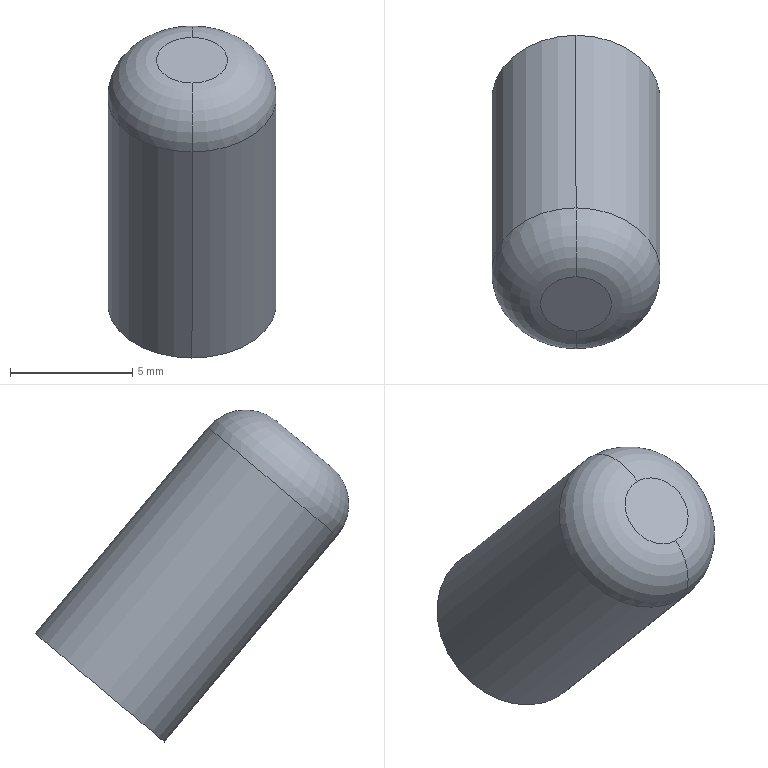Part | SolidWorks | features BaseBody 1 | 1 solid | 6 faces | box 6.9 x 12.824 x 13.576 mm | volume 469.908 mm3 | plane 2 | cylinder 2 | torus 2 | commonest cylinder face diameters 6.9 x2
STEP:
#1=CARTESIAN_POINT('',(-684.451,655.359,355.099));
#2=VERTEX_POINT('',#1);
#3=CARTESIAN_POINT('',(-684.451,660.644,359.534));
#4=VERTEX_POINT('',#3);
#5=CARTESIAN_POINT('',(-684.451,658.001,357.316));
#6=DIRECTION('',(0.000000993,-0.6428,0.766));
#7=DIRECTION('',(0.000001183,-0.766,-0.6428));
#8=AXIS2_PLACEMENT_3D('',#5,#6,#7);
#9=CIRCLE('',#8,3.45);
#10=EDGE_CURVE('',#2,#4,#9,.T.);
#11=ORIENTED_EDGE('',*,*,#10,.F.);
#12=CARTESIAN_POINT('',(-684.451,658.001,357.316));
#13=DIRECTION('',(0.000000993,-0.6428,0.766));
#14=DIRECTION('',(-0.000001183,0.766,0.6428));
#15=AXIS2_PLACEMENT_3D('',#12,#13,#14);
#16=CIRCLE('',#15,3.45);
#17=EDGE_CURVE('',#4,#2,#16,.T.);
#18=ORIENTED_EDGE('',*,*,#17,.F.);
#19=EDGE_LOOP('',(#11,#18));
#20=FACE_OUTER_BOUND('',#19,.T.);
#21=CARTESIAN_POINT('',(-750.729,655.382,355.118));
#22=DIRECTION('',(-0.000000993,0.6428,-0.766));
#23=DIRECTION('',(0.000001183,-0.766,-0.6428));
#24=AXIS2_PLACEMENT_3D('',#21,#22,#23);
#25=PLANE('',#24);
#26=ADVANCED_FACE('',(#20),#25,.T.);
#27=ORIENTED_EDGE('',*,*,#17,.T.);
#28=CARTESIAN_POINT('',(-684.451,648.288,363.525));
#29=VERTEX_POINT('',#28);
#30=CARTESIAN_POINT('',(-684.451,655.359,355.099));
#31=DIRECTION('',(0.000000993,-0.6428,0.766));
#32=VECTOR('',#31,1000.);
#33=LINE('',#30,#32);
#34=EDGE_CURVE('',#2,#29,#33,.T.);
#35=ORIENTED_EDGE('',*,*,#34,.T.);
#36=CARTESIAN_POINT('',(-684.451,653.574,367.96));
#37=VERTEX_POINT('',#36);
#38=CARTESIAN_POINT('',(-684.451,650.931,365.743));
#39=DIRECTION('',(-0.000000993,0.6428,-0.766));
#40=DIRECTION('',(0.000001183,-0.766,-0.6428));
#41=AXIS2_PLACEMENT_3D('',#38,#39,#40);
#42=CIRCLE('',#41,3.45);
#43=EDGE_CURVE('',#29,#37,#42,.T.);
#44=ORIENTED_EDGE('',*,*,#43,.T.);
#45=CARTESIAN_POINT('',(-684.451,653.574,367.96));
#46=DIRECTION('',(-0.000000993,0.6428,-0.766));
#47=VECTOR('',#46,1000.);
#48=LINE('',#45,#47);
#49=EDGE_CURVE('',#37,#4,#48,.T.);
#50=ORIENTED_EDGE('',*,*,#49,.T.);
#51=EDGE_LOOP('',(#27,#35,#44,#50));
#52=FACE_OUTER_BOUND('',#51,.T.);
#53=CARTESIAN_POINT('',(-684.451,658.001,357.316));
#54=DIRECTION('',(-0.000000993,0.6428,-0.766));
#55=DIRECTION('',(0.000001183,-0.766,-0.6428));
#56=AXIS2_PLACEMENT_3D('',#53,#54,#55);
#57=CYLINDRICAL_SURFACE('',#56,3.45);
#58=ADVANCED_FACE('',(#52),#57,.T.);
#59=ORIENTED_EDGE('',*,*,#10,.T.);
#60=ORIENTED_EDGE('',*,*,#49,.F.);
#61=CARTESIAN_POINT('',(-684.451,650.931,365.743));
#62=DIRECTION('',(-0.000000993,0.6428,-0.766));
#63=DIRECTION('',(-0.000001183,0.766,0.6428));
#64=AXIS2_PLACEMENT_3D('',#61,#62,#63);
#65=CIRCLE('',#64,3.45);
#66=EDGE_CURVE('',#37,#29,#65,.T.);
#67=ORIENTED_EDGE('',*,*,#66,.T.);
#68=ORIENTED_EDGE('',*,*,#34,.F.);
#69=EDGE_LOOP('',(#59,#60,#67,#68));
#70=FACE_OUTER_BOUND('',#69,.T.);
#71=CARTESIAN_POINT('',(-684.451,658.001,357.316));
#72=DIRECTION('',(-0.000000993,0.6428,-0.766));
#73=DIRECTION('',(0.000001183,-0.766,-0.6428));
#74=AXIS2_PLACEMENT_3D('',#71,#72,#73);
#75=CYLINDRICAL_SURFACE('',#74,3.45);
#76=ADVANCED_FACE('',(#70),#75,.T.);
#77=ORIENTED_EDGE('',*,*,#66,.F.);
#78=CARTESIAN_POINT('',(-684.451,650.756,368.207));
#79=VERTEX_POINT('',#78);
#80=CARTESIAN_POINT('',(-684.451,652.042,366.675));
#81=DIRECTION('',(-1.,-0.000001544,0.));
#82=DIRECTION('',(0.000000993,-0.6428,0.766));
#83=AXIS2_PLACEMENT_3D('',#80,#81,#82);
#84=CIRCLE('',#83,2.);
#85=EDGE_CURVE('',#79,#37,#84,.T.);
#86=ORIENTED_EDGE('',*,*,#85,.F.);
#87=CARTESIAN_POINT('',(-684.451,648.535,366.343));
#88=VERTEX_POINT('',#87);
#89=CARTESIAN_POINT('',(-684.451,649.645,367.275));
#90=DIRECTION('',(-0.000000993,0.6428,-0.766));
#91=DIRECTION('',(-0.000001183,0.766,0.6428));
#92=AXIS2_PLACEMENT_3D('',#89,#90,#91);
#93=CIRCLE('',#92,1.45);
#94=EDGE_CURVE('',#79,#88,#93,.T.);
#95=ORIENTED_EDGE('',*,*,#94,.T.);
#96=CARTESIAN_POINT('',(-684.451,649.82,364.811));
#97=DIRECTION('',(-1.,-0.000001544,0.));
#98=DIRECTION('',(0.000001183,-0.766,-0.6428));
#99=AXIS2_PLACEMENT_3D('',#96,#97,#98);
#100=CIRCLE('',#99,2.);
#101=EDGE_CURVE('',#29,#88,#100,.T.);
#102=ORIENTED_EDGE('',*,*,#101,.F.);
#103=EDGE_LOOP('',(#77,#86,#95,#102));
#104=FACE_OUTER_BOUND('',#103,.T.);
#105=CARTESIAN_POINT('',(-684.451,650.931,365.743));
#106=DIRECTION('',(-0.000000993,0.6428,-0.766));
#107=DIRECTION('',(-0.000001183,0.766,0.6428));
#108=AXIS2_PLACEMENT_3D('',#105,#106,#107);
#109=TOROIDAL_SURFACE('',#108,1.45,2.);
#110=ADVANCED_FACE('',(#104),#109,.T.);
#111=ORIENTED_EDGE('',*,*,#43,.F.);
#112=ORIENTED_EDGE('',*,*,#101,.T.);
#113=CARTESIAN_POINT('',(-684.451,649.645,367.275));
#114=DIRECTION('',(-0.000000993,0.6428,-0.766));
#115=DIRECTION('',(0.000001183,-0.766,-0.6428));
#116=AXIS2_PLACEMENT_3D('',#113,#114,#115);
#117=CIRCLE('',#116,1.45);
#118=EDGE_CURVE('',#88,#79,#117,.T.);
#119=ORIENTED_EDGE('',*,*,#118,.T.);
#120=ORIENTED_EDGE('',*,*,#85,.T.);
#121=EDGE_LOOP('',(#111,#112,#119,#120));
#122=FACE_OUTER_BOUND('',#121,.T.);
#123=CARTESIAN_POINT('',(-684.451,650.931,365.743));
#124=DIRECTION('',(-0.000000993,0.6428,-0.766));
#125=DIRECTION('',(-0.000001183,0.766,0.6428));
#126=AXIS2_PLACEMENT_3D('',#123,#124,#125);
#127=TOROIDAL_SURFACE('',#126,1.45,2.);
#128=ADVANCED_FACE('',(#122),#127,.T.);
#129=ORIENTED_EDGE('',*,*,#94,.F.);
#130=ORIENTED_EDGE('',*,*,#118,.F.);
#131=EDGE_LOOP('',(#129,#130));
#132=FACE_OUTER_BOUND('',#131,.T.);
#133=CARTESIAN_POINT('',(-750.729,647.025,365.077));
#134=DIRECTION('',(-0.000000993,0.6428,-0.766));
#135=DIRECTION('',(0.000001183,-0.766,-0.6428));
#136=AXIS2_PLACEMENT_3D('',#133,#134,#135);
#137=PLANE('',#136);
#138=ADVANCED_FACE('',(#132),#137,.F.);
#139=CLOSED_SHELL('',(#26,#58,#76,#110,#128,#138));
#140=MANIFOLD_SOLID_BREP('',#139);
#141=CARTESIAN_POINT('',(0.,0.,0.));
#142=DIRECTION('',(0.,0.,1.));
#143=DIRECTION('',(1.,0.,0.));
#144=AXIS2_PLACEMENT_3D('',#141,#142,#143);
#145=(LENGTH_UNIT()NAMED_UNIT(*)SI_UNIT(.MILLI.,.METRE.));
#146=UNCERTAINTY_MEASURE_WITH_UNIT(LENGTH_MEASURE(0.00001),#145,'','');
#147=(NAMED_UNIT(*)PLANE_ANGLE_UNIT()SI_UNIT($,.RADIAN.));
#148=(NAMED_UNIT(*)SI_UNIT($,.STERADIAN.)SOLID_ANGLE_UNIT());
#149=(GEOMETRIC_REPRESENTATION_CONTEXT(3)GLOBAL_UNCERTAINTY_ASSIGNED_CONTEXT((#146))GLOBAL_UNIT_ASSIGNED_CONTEXT((#145,#147,#148))REPRESENTATION_CONTEXT('',''));
#150=ADVANCED_BREP_SHAPE_REPRESENTATION('',(#140,#144),#149);